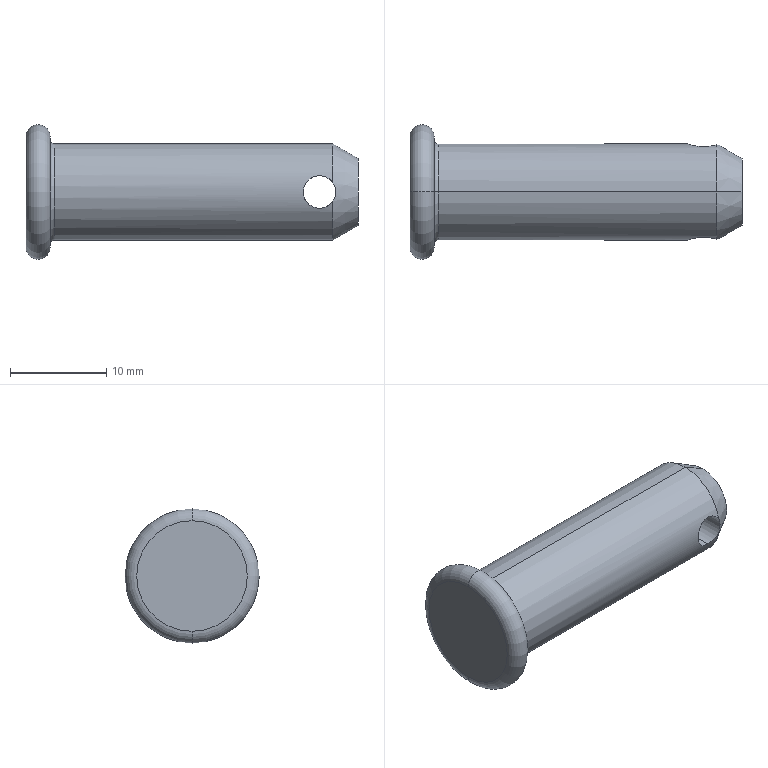Part | SolidWorks | features Chamfer 1, Cut 1, Fillet 1, Revolution 1 | 1 solid | 13 faces | box 34.5 x 14 x 14 mm | volume 2728 mm3 | cylinder 4 | torus 4 | plane 3 | cone 2 | commonest cylinder face diameters 3.38 x2 10 x2
STEP:
#1=CARTESIAN_POINT('',(30.5,-4.706,-1.69));
#2=VERTEX_POINT('',#1);
#3=CARTESIAN_POINT('',(30.5,-4.706,1.69));
#4=VERTEX_POINT('',#3);
#5=CARTESIAN_POINT('',(30.5,-4.706,-1.69));
#6=CARTESIAN_POINT('',(30.276,-4.706,-1.69));
#7=CARTESIAN_POINT('',(30.055,-4.722,-1.645));
#8=CARTESIAN_POINT('',(29.747,-4.765,-1.517));
#9=CARTESIAN_POINT('',(29.65,-4.781,-1.465));
#10=CARTESIAN_POINT('',(29.468,-4.817,-1.343));
#11=CARTESIAN_POINT('',(29.382,-4.836,-1.272));
#12=CARTESIAN_POINT('',(29.15,-4.893,-1.039));
#13=CARTESIAN_POINT('',(29.024,-4.931,-0.8522));
#14=CARTESIAN_POINT('',(28.855,-4.984,-0.4461));
#15=CARTESIAN_POINT('',(28.81,-5.,-0.2222));
#16=CARTESIAN_POINT('',(28.81,-5.,0.1106));
#17=CARTESIAN_POINT('',(28.821,-4.996,0.2234));
#18=CARTESIAN_POINT('',(28.865,-4.982,0.4413));
#19=CARTESIAN_POINT('',(28.897,-4.971,0.547));
#20=CARTESIAN_POINT('',(29.025,-4.931,0.8543));
#21=CARTESIAN_POINT('',(29.149,-4.893,1.04));
#22=CARTESIAN_POINT('',(29.384,-4.836,1.274));
#23=CARTESIAN_POINT('',(29.468,-4.817,1.343));
#24=CARTESIAN_POINT('',(29.65,-4.781,1.465));
#25=CARTESIAN_POINT('',(29.749,-4.764,1.518));
#26=CARTESIAN_POINT('',(29.953,-4.736,1.603));
#27=CARTESIAN_POINT('',(30.058,-4.725,1.635));
#28=CARTESIAN_POINT('',(30.276,-4.71,1.679));
#29=CARTESIAN_POINT('',(30.389,-4.706,1.69));
#30=CARTESIAN_POINT('',(30.5,-4.706,1.69));
#31=B_SPLINE_CURVE_WITH_KNOTS('',3,(#5,#6,#7,#8,#9,#10,#11,#12,#13,#14,#15,#16,#17,#18,#19,#20,#21,#22,#23,#24,#25,#26,#27,#28,#29,#30),.UNSPECIFIED.,.F.,.F.,(4,2,2,2,2,2,2,2,2,2,2,2,4),(0.001661,0.002326,0.002659,0.002992,0.003657,0.004322,0.004654,0.004987,0.005652,0.005985,0.006317,0.00665,0.006982),.UNSPECIFIED.);
#32=EDGE_CURVE('',#2,#4,#31,.T.);
#33=ORIENTED_EDGE('',*,*,#32,.F.);
#34=CARTESIAN_POINT('',(30.5,4.706,-1.69));
#35=VERTEX_POINT('',#34);
#36=CARTESIAN_POINT('',(30.5,-500.,-1.69));
#37=DIRECTION('',(0.,1.,0.));
#38=VECTOR('',#37,1000.);
#39=LINE('',#36,#38);
#40=EDGE_CURVE('',#2,#35,#39,.T.);
#41=ORIENTED_EDGE('',*,*,#40,.T.);
#42=CARTESIAN_POINT('',(30.5,4.706,1.69));
#43=VERTEX_POINT('',#42);
#44=CARTESIAN_POINT('',(30.5,4.706,1.69));
#45=CARTESIAN_POINT('',(30.276,4.706,1.69));
#46=CARTESIAN_POINT('',(30.055,4.722,1.645));
#47=CARTESIAN_POINT('',(29.747,4.765,1.517));
#48=CARTESIAN_POINT('',(29.65,4.781,1.465));
#49=CARTESIAN_POINT('',(29.468,4.817,1.343));
#50=CARTESIAN_POINT('',(29.382,4.836,1.272));
#51=CARTESIAN_POINT('',(29.15,4.893,1.039));
#52=CARTESIAN_POINT('',(29.024,4.931,0.8522));
#53=CARTESIAN_POINT('',(28.855,4.984,0.4461));
#54=CARTESIAN_POINT('',(28.81,5.,0.2222));
#55=CARTESIAN_POINT('',(28.81,5.,-0.1106));
#56=CARTESIAN_POINT('',(28.821,4.996,-0.2234));
#57=CARTESIAN_POINT('',(28.865,4.982,-0.4413));
#58=CARTESIAN_POINT('',(28.897,4.971,-0.547));
#59=CARTESIAN_POINT('',(29.025,4.931,-0.8543));
#60=CARTESIAN_POINT('',(29.149,4.893,-1.04));
#61=CARTESIAN_POINT('',(29.384,4.836,-1.274));
#62=CARTESIAN_POINT('',(29.468,4.817,-1.343));
#63=CARTESIAN_POINT('',(29.65,4.781,-1.465));
#64=CARTESIAN_POINT('',(29.749,4.764,-1.518));
#65=CARTESIAN_POINT('',(29.953,4.736,-1.603));
#66=CARTESIAN_POINT('',(30.058,4.725,-1.635));
#67=CARTESIAN_POINT('',(30.276,4.71,-1.679));
#68=CARTESIAN_POINT('',(30.389,4.706,-1.69));
#69=CARTESIAN_POINT('',(30.5,4.706,-1.69));
#70=B_SPLINE_CURVE_WITH_KNOTS('',3,(#44,#45,#46,#47,#48,#49,#50,#51,#52,#53,#54,#55,#56,#57,#58,#59,#60,#61,#62,#63,#64,#65,#66,#67,#68,#69),.UNSPECIFIED.,.F.,.F.,(4,2,2,2,2,2,2,2,2,2,2,2,4),(0.001661,0.002326,0.002659,0.002992,0.003657,0.004322,0.004654,0.004987,0.005652,0.005985,0.006317,0.00665,0.006982),.UNSPECIFIED.);
#71=EDGE_CURVE('',#43,#35,#70,.T.);
#72=ORIENTED_EDGE('',*,*,#71,.F.);
#73=CARTESIAN_POINT('',(30.5,-500.,1.69));
#74=DIRECTION('',(0.,1.,0.));
#75=VECTOR('',#74,1000.);
#76=LINE('',#73,#75);
#77=EDGE_CURVE('',#4,#43,#76,.T.);
#78=ORIENTED_EDGE('',*,*,#77,.F.);
#79=EDGE_LOOP('',(#33,#41,#72,#78));
#80=FACE_OUTER_BOUND('',#79,.T.);
#81=CARTESIAN_POINT('',(30.5,-500.,0.));
#82=DIRECTION('',(0.,1.,0.));
#83=DIRECTION('',(0.,0.,1.));
#84=AXIS2_PLACEMENT_3D('',#81,#82,#83);
#85=CYLINDRICAL_SURFACE('',#84,1.69);
#86=ADVANCED_FACE('',(#80),#85,.F.);
#87=CARTESIAN_POINT('',(34.5,0.,-3.5));
#88=VERTEX_POINT('',#87);
#89=CARTESIAN_POINT('',(34.5,0.,3.5));
#90=VERTEX_POINT('',#89);
#91=CARTESIAN_POINT('',(34.5,0.,0.));
#92=DIRECTION('',(1.,0.,0.));
#93=DIRECTION('',(0.,0.,1.));
#94=AXIS2_PLACEMENT_3D('',#91,#92,#93);
#95=CIRCLE('',#94,3.5);
#96=EDGE_CURVE('',#88,#90,#95,.T.);
#97=ORIENTED_EDGE('',*,*,#96,.F.);
#98=CARTESIAN_POINT('',(31.902,0.,-5.));
#99=VERTEX_POINT('',#98);
#100=CARTESIAN_POINT('',(31.902,0.,-5.));
#101=DIRECTION('',(-0.866,0.,-0.5));
#102=VECTOR('',#101,1000.);
#103=LINE('',#100,#102);
#104=EDGE_CURVE('',#88,#99,#103,.T.);
#105=ORIENTED_EDGE('',*,*,#104,.T.);
#106=CARTESIAN_POINT('',(31.902,4.91,-0.9438));
#107=VERTEX_POINT('',#106);
#108=CARTESIAN_POINT('',(31.902,0.,0.));
#109=DIRECTION('',(-1.,0.,0.));
#110=DIRECTION('',(0.,0.,1.));
#111=AXIS2_PLACEMENT_3D('',#108,#109,#110);
#112=CIRCLE('',#111,5.);
#113=EDGE_CURVE('',#107,#99,#112,.T.);
#114=ORIENTED_EDGE('',*,*,#113,.F.);
#115=CARTESIAN_POINT('',(31.902,4.91,0.9438));
#116=VERTEX_POINT('',#115);
#117=CARTESIAN_POINT('',(31.902,4.91,0.9438));
#118=CARTESIAN_POINT('',(31.995,4.882,0.8061));
#119=CARTESIAN_POINT('',(32.066,4.864,0.6567));
#120=CARTESIAN_POINT('',(32.165,4.839,0.3342));
#121=CARTESIAN_POINT('',(32.19,4.834,0.1694));
#122=CARTESIAN_POINT('',(32.19,4.834,-0.1673));
#123=CARTESIAN_POINT('',(32.165,4.839,-0.3337));
#124=CARTESIAN_POINT('',(32.067,4.863,-0.6536));
#125=CARTESIAN_POINT('',(31.995,4.882,-0.806));
#126=CARTESIAN_POINT('',(31.902,4.91,-0.9438));
#127=B_SPLINE_CURVE_WITH_KNOTS('',3,(#117,#118,#119,#120,#121,#122,#123,#124,#125,#126),.UNSPECIFIED.,.F.,.F.,(4,2,2,2,4),(0.00005098,0.0005511,0.001051,0.001551,0.002051),.UNSPECIFIED.);
#128=EDGE_CURVE('',#116,#107,#127,.T.);
#129=ORIENTED_EDGE('',*,*,#128,.F.);
#130=CARTESIAN_POINT('',(31.902,0.,5.));
#131=VERTEX_POINT('',#130);
#132=CARTESIAN_POINT('',(31.902,0.,0.));
#133=DIRECTION('',(-1.,0.,0.));
#134=DIRECTION('',(0.,0.,1.));
#135=AXIS2_PLACEMENT_3D('',#132,#133,#134);
#136=CIRCLE('',#135,5.);
#137=EDGE_CURVE('',#131,#116,#136,.T.);
#138=ORIENTED_EDGE('',*,*,#137,.F.);
#139=CARTESIAN_POINT('',(31.902,0.,5.));
#140=DIRECTION('',(-0.866,0.,0.5));
#141=VECTOR('',#140,1000.);
#142=LINE('',#139,#141);
#143=EDGE_CURVE('',#90,#131,#142,.T.);
#144=ORIENTED_EDGE('',*,*,#143,.F.);
#145=EDGE_LOOP('',(#97,#105,#114,#129,#138,#144));
#146=FACE_OUTER_BOUND('',#145,.T.);
#147=CARTESIAN_POINT('',(31.902,0.,0.));
#148=DIRECTION('',(-1.,0.,0.));
#149=DIRECTION('',(0.,0.,1.));
#150=AXIS2_PLACEMENT_3D('',#147,#148,#149);
#151=CONICAL_SURFACE('',#150,5.,0.5236);
#152=ADVANCED_FACE('',(#146),#151,.T.);
#153=CARTESIAN_POINT('',(2.5,0.,-5.5));
#154=VERTEX_POINT('',#153);
#155=CARTESIAN_POINT('',(2.5,0.,5.5));
#156=VERTEX_POINT('',#155);
#157=CARTESIAN_POINT('',(2.5,0.,0.));
#158=DIRECTION('',(-1.,0.,0.));
#159=DIRECTION('',(0.,0.,1.));
#160=AXIS2_PLACEMENT_3D('',#157,#158,#159);
#161=CIRCLE('',#160,5.5);
#162=EDGE_CURVE('',#154,#156,#161,.T.);
#163=ORIENTED_EDGE('',*,*,#162,.F.);
#164=CARTESIAN_POINT('',(3.,0.,-5.));
#165=VERTEX_POINT('',#164);
#166=CARTESIAN_POINT('',(3.,0.,-5.5));
#167=DIRECTION('',(0.,1.,0.));
#168=DIRECTION('',(0.,0.,1.));
#169=AXIS2_PLACEMENT_3D('',#166,#167,#168);
#170=CIRCLE('',#169,0.5);
#171=EDGE_CURVE('',#154,#165,#170,.T.);
#172=ORIENTED_EDGE('',*,*,#171,.T.);
#173=CARTESIAN_POINT('',(3.,0.,5.));
#174=VERTEX_POINT('',#173);
#175=CARTESIAN_POINT('',(3.,0.,0.));
#176=DIRECTION('',(1.,0.,0.));
#177=DIRECTION('',(0.,0.,1.));
#178=AXIS2_PLACEMENT_3D('',#175,#176,#177);
#179=CIRCLE('',#178,5.);
#180=EDGE_CURVE('',#174,#165,#179,.T.);
#181=ORIENTED_EDGE('',*,*,#180,.F.);
#182=CARTESIAN_POINT('',(3.,0.,5.5));
#183=DIRECTION('',(0.,-1.,0.));
#184=DIRECTION('',(0.,0.,-1.));
#185=AXIS2_PLACEMENT_3D('',#182,#183,#184);
#186=CIRCLE('',#185,0.5);
#187=EDGE_CURVE('',#156,#174,#186,.T.);
#188=ORIENTED_EDGE('',*,*,#187,.F.);
#189=EDGE_LOOP('',(#163,#172,#181,#188));
#190=FACE_OUTER_BOUND('',#189,.T.);
#191=CARTESIAN_POINT('',(3.,0.,0.));
#192=DIRECTION('',(-1.,0.,0.));
#193=DIRECTION('',(0.,0.,1.));
#194=AXIS2_PLACEMENT_3D('',#191,#192,#193);
#195=TOROIDAL_SURFACE('',#194,5.5,0.5);
#196=ADVANCED_FACE('',(#190),#195,.F.);
#197=ORIENTED_EDGE('',*,*,#113,.T.);
#198=CARTESIAN_POINT('',(0.,0.,-5.));
#199=DIRECTION('',(-1.,0.,0.));
#200=VECTOR('',#199,1000.);
#201=LINE('',#198,#200);
#202=EDGE_CURVE('',#99,#165,#201,.T.);
#203=ORIENTED_EDGE('',*,*,#202,.T.);
#204=CARTESIAN_POINT('',(3.,0.,0.));
#205=DIRECTION('',(1.,0.,0.));
#206=DIRECTION('',(0.,0.,1.));
#207=AXIS2_PLACEMENT_3D('',#204,#205,#206);
#208=CIRCLE('',#207,5.);
#209=EDGE_CURVE('',#165,#174,#208,.T.);
#210=ORIENTED_EDGE('',*,*,#209,.T.);
#211=CARTESIAN_POINT('',(0.,0.,5.));
#212=DIRECTION('',(-1.,0.,0.));
#213=VECTOR('',#212,1000.);
#214=LINE('',#211,#213);
#215=EDGE_CURVE('',#131,#174,#214,.T.);
#216=ORIENTED_EDGE('',*,*,#215,.F.);
#217=ORIENTED_EDGE('',*,*,#137,.T.);
#218=CARTESIAN_POINT('',(31.902,4.91,0.9438));
#219=CARTESIAN_POINT('',(31.824,4.888,1.059));
#220=CARTESIAN_POINT('',(31.735,4.864,1.162));
#221=CARTESIAN_POINT('',(31.532,4.817,1.345));
#222=CARTESIAN_POINT('',(31.418,4.793,1.426));
#223=CARTESIAN_POINT('',(31.176,4.753,1.555));
#224=CARTESIAN_POINT('',(31.046,4.735,1.605));
#225=CARTESIAN_POINT('',(30.777,4.712,1.673));
#226=CARTESIAN_POINT('',(30.64,4.706,1.69));
#227=CARTESIAN_POINT('',(30.5,4.706,1.69));
#228=B_SPLINE_CURVE_WITH_KNOTS('',3,(#218,#219,#220,#221,#222,#223,#224,#225,#226,#227),.UNSPECIFIED.,.F.,.F.,(4,2,2,2,4),(0.,0.0004153,0.0008306,0.001246,0.001661),.UNSPECIFIED.);
#229=EDGE_CURVE('',#116,#43,#228,.T.);
#230=ORIENTED_EDGE('',*,*,#229,.T.);
#231=ORIENTED_EDGE('',*,*,#71,.T.);
#232=CARTESIAN_POINT('',(30.5,4.706,-1.69));
#233=CARTESIAN_POINT('',(30.638,4.706,-1.69));
#234=CARTESIAN_POINT('',(30.777,4.712,-1.673));
#235=CARTESIAN_POINT('',(31.047,4.735,-1.605));
#236=CARTESIAN_POINT('',(31.175,4.752,-1.556));
#237=CARTESIAN_POINT('',(31.54,4.813,-1.36));
#238=CARTESIAN_POINT('',(31.747,4.866,-1.173));
#239=CARTESIAN_POINT('',(31.902,4.91,-0.9438));
#240=B_SPLINE_CURVE_WITH_KNOTS('',3,(#232,#233,#234,#235,#236,#237,#238,#239),.UNSPECIFIED.,.F.,.F.,(4,2,2,4),(0.006982,0.007397,0.007811,0.00864),.UNSPECIFIED.);
#241=EDGE_CURVE('',#35,#107,#240,.T.);
#242=ORIENTED_EDGE('',*,*,#241,.T.);
#243=EDGE_LOOP('',(#197,#203,#210,#216,#217,#230,#231,#242));
#244=FACE_OUTER_BOUND('',#243,.T.);
#245=CARTESIAN_POINT('',(0.,0.,0.));
#246=DIRECTION('',(-1.,0.,0.));
#247=DIRECTION('',(0.,0.,1.));
#248=AXIS2_PLACEMENT_3D('',#245,#246,#247);
#249=CYLINDRICAL_SURFACE('',#248,5.);
#250=ADVANCED_FACE('',(#244),#249,.T.);
#251=CARTESIAN_POINT('',(2.5,0.,5.75));
#252=VERTEX_POINT('',#251);
#253=CARTESIAN_POINT('',(2.5,0.,-5.75));
#254=VERTEX_POINT('',#253);
#255=CARTESIAN_POINT('',(2.5,0.,0.));
#256=DIRECTION('',(-1.,0.,0.));
#257=DIRECTION('',(0.,0.,1.));
#258=AXIS2_PLACEMENT_3D('',#255,#256,#257);
#259=CIRCLE('',#258,5.75);
#260=EDGE_CURVE('',#252,#254,#259,.T.);
#261=ORIENTED_EDGE('',*,*,#260,.T.);
#262=CARTESIAN_POINT('',(0.,0.,-5.75));
#263=VERTEX_POINT('',#262);
#264=CARTESIAN_POINT('',(1.25,0.,-5.75));
#265=DIRECTION('',(0.,1.,0.));
#266=DIRECTION('',(0.,0.,1.));
#267=AXIS2_PLACEMENT_3D('',#264,#265,#266);
#268=CIRCLE('',#267,1.25);
#269=EDGE_CURVE('',#254,#263,#268,.T.);
#270=ORIENTED_EDGE('',*,*,#269,.T.);
#271=CARTESIAN_POINT('',(0.,0.,5.75));
#272=VERTEX_POINT('',#271);
#273=CARTESIAN_POINT('',(0.,0.,0.));
#274=DIRECTION('',(-1.,0.,0.));
#275=DIRECTION('',(0.,0.,1.));
#276=AXIS2_PLACEMENT_3D('',#273,#274,#275);
#277=CIRCLE('',#276,5.75);
#278=EDGE_CURVE('',#272,#263,#277,.T.);
#279=ORIENTED_EDGE('',*,*,#278,.F.);
#280=CARTESIAN_POINT('',(1.25,0.,5.75));
#281=DIRECTION('',(0.,-1.,0.));
#282=DIRECTION('',(0.,0.,-1.));
#283=AXIS2_PLACEMENT_3D('',#280,#281,#282);
#284=CIRCLE('',#283,1.25);
#285=EDGE_CURVE('',#252,#272,#284,.T.);
#286=ORIENTED_EDGE('',*,*,#285,.F.);
#287=EDGE_LOOP('',(#261,#270,#279,#286));
#288=FACE_OUTER_BOUND('',#287,.T.);
#289=CARTESIAN_POINT('',(1.25,0.,0.));
#290=DIRECTION('',(-1.,0.,0.));
#291=DIRECTION('',(0.,0.,1.));
#292=AXIS2_PLACEMENT_3D('',#289,#290,#291);
#293=TOROIDAL_SURFACE('',#292,5.75,1.25);
#294=ADVANCED_FACE('',(#288),#293,.T.);
#295=ORIENTED_EDGE('',*,*,#278,.T.);
#296=CARTESIAN_POINT('',(0.,0.,0.));
#297=DIRECTION('',(-1.,0.,0.));
#298=DIRECTION('',(0.,0.,1.));
#299=AXIS2_PLACEMENT_3D('',#296,#297,#298);
#300=CIRCLE('',#299,5.75);
#301=EDGE_CURVE('',#263,#272,#300,.T.);
#302=ORIENTED_EDGE('',*,*,#301,.T.);
#303=EDGE_LOOP('',(#295,#302));
#304=FACE_OUTER_BOUND('',#303,.T.);
#305=CARTESIAN_POINT('',(0.,0.,0.));
#306=DIRECTION('',(1.,0.,0.));
#307=DIRECTION('',(0.,0.,-1.));
#308=AXIS2_PLACEMENT_3D('',#305,#306,#307);
#309=PLANE('',#308);
#310=ADVANCED_FACE('',(#304),#309,.F.);
#311=ORIENTED_EDGE('',*,*,#269,.F.);
#312=CARTESIAN_POINT('',(2.5,0.,0.));
#313=DIRECTION('',(-1.,0.,0.));
#314=DIRECTION('',(0.,0.,1.));
#315=AXIS2_PLACEMENT_3D('',#312,#313,#314);
#316=CIRCLE('',#315,5.75);
#317=EDGE_CURVE('',#254,#252,#316,.T.);
#318=ORIENTED_EDGE('',*,*,#317,.T.);
#319=ORIENTED_EDGE('',*,*,#285,.T.);
#320=ORIENTED_EDGE('',*,*,#301,.F.);
#321=EDGE_LOOP('',(#311,#318,#319,#320));
#322=FACE_OUTER_BOUND('',#321,.T.);
#323=CARTESIAN_POINT('',(1.25,0.,0.));
#324=DIRECTION('',(-1.,0.,0.));
#325=DIRECTION('',(0.,0.,1.));
#326=AXIS2_PLACEMENT_3D('',#323,#324,#325);
#327=TOROIDAL_SURFACE('',#326,5.75,1.25);
#328=ADVANCED_FACE('',(#322),#327,.T.);
#329=CARTESIAN_POINT('',(2.5,0.,0.));
#330=DIRECTION('',(-1.,0.,0.));
#331=DIRECTION('',(0.,0.,1.));
#332=AXIS2_PLACEMENT_3D('',#329,#330,#331);
#333=CIRCLE('',#332,5.5);
#334=EDGE_CURVE('',#156,#154,#333,.T.);
#335=ORIENTED_EDGE('',*,*,#334,.T.);
#336=ORIENTED_EDGE('',*,*,#162,.T.);
#337=EDGE_LOOP('',(#335,#336));
#338=FACE_BOUND('',#337,.T.);
#339=ORIENTED_EDGE('',*,*,#260,.F.);
#340=ORIENTED_EDGE('',*,*,#317,.F.);
#341=EDGE_LOOP('',(#339,#340));
#342=FACE_OUTER_BOUND('',#341,.T.);
#343=CARTESIAN_POINT('',(2.5,5.75,0.));
#344=DIRECTION('',(-1.,0.,0.));
#345=DIRECTION('',(0.,0.,1.));
#346=AXIS2_PLACEMENT_3D('',#343,#344,#345);
#347=PLANE('',#346);
#348=ADVANCED_FACE('',(#338,#342),#347,.F.);
#349=ORIENTED_EDGE('',*,*,#202,.F.);
#350=CARTESIAN_POINT('',(31.902,-4.91,-0.9438));
#351=VERTEX_POINT('',#350);
#352=CARTESIAN_POINT('',(31.902,0.,0.));
#353=DIRECTION('',(-1.,0.,0.));
#354=DIRECTION('',(0.,0.,1.));
#355=AXIS2_PLACEMENT_3D('',#352,#353,#354);
#356=CIRCLE('',#355,5.);
#357=EDGE_CURVE('',#99,#351,#356,.T.);
#358=ORIENTED_EDGE('',*,*,#357,.T.);
#359=CARTESIAN_POINT('',(31.902,-4.91,-0.9438));
#360=CARTESIAN_POINT('',(31.824,-4.888,-1.059));
#361=CARTESIAN_POINT('',(31.735,-4.864,-1.162));
#362=CARTESIAN_POINT('',(31.532,-4.817,-1.345));
#363=CARTESIAN_POINT('',(31.418,-4.793,-1.426));
#364=CARTESIAN_POINT('',(31.176,-4.753,-1.555));
#365=CARTESIAN_POINT('',(31.046,-4.735,-1.605));
#366=CARTESIAN_POINT('',(30.777,-4.712,-1.673));
#367=CARTESIAN_POINT('',(30.64,-4.706,-1.69));
#368=CARTESIAN_POINT('',(30.5,-4.706,-1.69));
#369=B_SPLINE_CURVE_WITH_KNOTS('',3,(#359,#360,#361,#362,#363,#364,#365,#366,#367,#368),.UNSPECIFIED.,.F.,.F.,(4,2,2,2,4),(0.,0.0004153,0.0008306,0.001246,0.001661),.UNSPECIFIED.);
#370=EDGE_CURVE('',#351,#2,#369,.T.);
#371=ORIENTED_EDGE('',*,*,#370,.T.);
#372=ORIENTED_EDGE('',*,*,#32,.T.);
#373=CARTESIAN_POINT('',(31.902,-4.91,0.9438));
#374=VERTEX_POINT('',#373);
#375=CARTESIAN_POINT('',(30.5,-4.706,1.69));
#376=CARTESIAN_POINT('',(30.638,-4.706,1.69));
#377=CARTESIAN_POINT('',(30.777,-4.712,1.673));
#378=CARTESIAN_POINT('',(31.047,-4.735,1.605));
#379=CARTESIAN_POINT('',(31.175,-4.752,1.556));
#380=CARTESIAN_POINT('',(31.54,-4.813,1.36));
#381=CARTESIAN_POINT('',(31.747,-4.866,1.173));
#382=CARTESIAN_POINT('',(31.902,-4.91,0.9438));
#383=B_SPLINE_CURVE_WITH_KNOTS('',3,(#375,#376,#377,#378,#379,#380,#381,#382),.UNSPECIFIED.,.F.,.F.,(4,2,2,4),(0.006982,0.007397,0.007811,0.00864),.UNSPECIFIED.);
#384=EDGE_CURVE('',#4,#374,#383,.T.);
#385=ORIENTED_EDGE('',*,*,#384,.T.);
#386=CARTESIAN_POINT('',(31.902,0.,0.));
#387=DIRECTION('',(-1.,0.,0.));
#388=DIRECTION('',(0.,0.,1.));
#389=AXIS2_PLACEMENT_3D('',#386,#387,#388);
#390=CIRCLE('',#389,5.);
#391=EDGE_CURVE('',#374,#131,#390,.T.);
#392=ORIENTED_EDGE('',*,*,#391,.T.);
#393=ORIENTED_EDGE('',*,*,#215,.T.);
#394=ORIENTED_EDGE('',*,*,#180,.T.);
#395=EDGE_LOOP('',(#349,#358,#371,#372,#385,#392,#393,#394));
#396=FACE_OUTER_BOUND('',#395,.T.);
#397=CARTESIAN_POINT('',(0.,0.,0.));
#398=DIRECTION('',(-1.,0.,0.));
#399=DIRECTION('',(0.,0.,1.));
#400=AXIS2_PLACEMENT_3D('',#397,#398,#399);
#401=CYLINDRICAL_SURFACE('',#400,5.);
#402=ADVANCED_FACE('',(#396),#401,.T.);
#403=CARTESIAN_POINT('',(34.5,0.,0.));
#404=DIRECTION('',(1.,0.,0.));
#405=DIRECTION('',(0.,0.,1.));
#406=AXIS2_PLACEMENT_3D('',#403,#404,#405);
#407=CIRCLE('',#406,3.5);
#408=EDGE_CURVE('',#90,#88,#407,.T.);
#409=ORIENTED_EDGE('',*,*,#408,.T.);
#410=ORIENTED_EDGE('',*,*,#96,.T.);
#411=EDGE_LOOP('',(#409,#410));
#412=FACE_OUTER_BOUND('',#411,.T.);
#413=CARTESIAN_POINT('',(34.5,5.,0.));
#414=DIRECTION('',(-1.,0.,0.));
#415=DIRECTION('',(0.,0.,1.));
#416=AXIS2_PLACEMENT_3D('',#413,#414,#415);
#417=PLANE('',#416);
#418=ADVANCED_FACE('',(#412),#417,.F.);
#419=ORIENTED_EDGE('',*,*,#171,.F.);
#420=ORIENTED_EDGE('',*,*,#334,.F.);
#421=ORIENTED_EDGE('',*,*,#187,.T.);
#422=ORIENTED_EDGE('',*,*,#209,.F.);
#423=EDGE_LOOP('',(#419,#420,#421,#422));
#424=FACE_OUTER_BOUND('',#423,.T.);
#425=CARTESIAN_POINT('',(3.,0.,0.));
#426=DIRECTION('',(-1.,0.,0.));
#427=DIRECTION('',(0.,0.,1.));
#428=AXIS2_PLACEMENT_3D('',#425,#426,#427);
#429=TOROIDAL_SURFACE('',#428,5.5,0.5);
#430=ADVANCED_FACE('',(#424),#429,.F.);
#431=ORIENTED_EDGE('',*,*,#104,.F.);
#432=ORIENTED_EDGE('',*,*,#408,.F.);
#433=ORIENTED_EDGE('',*,*,#143,.T.);
#434=ORIENTED_EDGE('',*,*,#391,.F.);
#435=CARTESIAN_POINT('',(31.902,-4.91,-0.9438));
#436=CARTESIAN_POINT('',(31.995,-4.882,-0.8061));
#437=CARTESIAN_POINT('',(32.066,-4.864,-0.6567));
#438=CARTESIAN_POINT('',(32.165,-4.839,-0.3342));
#439=CARTESIAN_POINT('',(32.19,-4.834,-0.1694));
#440=CARTESIAN_POINT('',(32.19,-4.834,0.1673));
#441=CARTESIAN_POINT('',(32.165,-4.839,0.3337));
#442=CARTESIAN_POINT('',(32.067,-4.863,0.6536));
#443=CARTESIAN_POINT('',(31.995,-4.882,0.806));
#444=CARTESIAN_POINT('',(31.902,-4.91,0.9438));
#445=B_SPLINE_CURVE_WITH_KNOTS('',3,(#435,#436,#437,#438,#439,#440,#441,#442,#443,#444),.UNSPECIFIED.,.F.,.F.,(4,2,2,2,4),(0.00005098,0.0005511,0.001051,0.001551,0.002051),.UNSPECIFIED.);
#446=EDGE_CURVE('',#351,#374,#445,.T.);
#447=ORIENTED_EDGE('',*,*,#446,.F.);
#448=ORIENTED_EDGE('',*,*,#357,.F.);
#449=EDGE_LOOP('',(#431,#432,#433,#434,#447,#448));
#450=FACE_OUTER_BOUND('',#449,.T.);
#451=CARTESIAN_POINT('',(31.902,0.,0.));
#452=DIRECTION('',(-1.,0.,0.));
#453=DIRECTION('',(0.,0.,1.));
#454=AXIS2_PLACEMENT_3D('',#451,#452,#453);
#455=CONICAL_SURFACE('',#454,5.,0.5236);
#456=ADVANCED_FACE('',(#450),#455,.T.);
#457=ORIENTED_EDGE('',*,*,#40,.F.);
#458=ORIENTED_EDGE('',*,*,#370,.F.);
#459=ORIENTED_EDGE('',*,*,#446,.T.);
#460=ORIENTED_EDGE('',*,*,#384,.F.);
#461=ORIENTED_EDGE('',*,*,#77,.T.);
#462=ORIENTED_EDGE('',*,*,#229,.F.);
#463=ORIENTED_EDGE('',*,*,#128,.T.);
#464=ORIENTED_EDGE('',*,*,#241,.F.);
#465=EDGE_LOOP('',(#457,#458,#459,#460,#461,#462,#463,#464));
#466=FACE_OUTER_BOUND('',#465,.T.);
#467=CARTESIAN_POINT('',(30.5,-500.,0.));
#468=DIRECTION('',(0.,1.,0.));
#469=DIRECTION('',(0.,0.,1.));
#470=AXIS2_PLACEMENT_3D('',#467,#468,#469);
#471=CYLINDRICAL_SURFACE('',#470,1.69);
#472=ADVANCED_FACE('',(#466),#471,.F.);
#473=CLOSED_SHELL('',(#86,#152,#196,#250,#294,#310,#328,#348,#402,#418,#430,#456,#472));
#474=MANIFOLD_SOLID_BREP('',#473);
#475=CARTESIAN_POINT('',(0.,0.,0.));
#476=DIRECTION('',(0.,0.,1.));
#477=DIRECTION('',(1.,0.,0.));
#478=AXIS2_PLACEMENT_3D('',#475,#476,#477);
#479=(LENGTH_UNIT()NAMED_UNIT(*)SI_UNIT(.MILLI.,.METRE.));
#480=UNCERTAINTY_MEASURE_WITH_UNIT(LENGTH_MEASURE(0.00001),#479,'','');
#481=(NAMED_UNIT(*)PLANE_ANGLE_UNIT()SI_UNIT($,.RADIAN.));
#482=(NAMED_UNIT(*)SI_UNIT($,.STERADIAN.)SOLID_ANGLE_UNIT());
#483=(GEOMETRIC_REPRESENTATION_CONTEXT(3)GLOBAL_UNCERTAINTY_ASSIGNED_CONTEXT((#480))GLOBAL_UNIT_ASSIGNED_CONTEXT((#479,#481,#482))REPRESENTATION_CONTEXT('',''));
#484=ADVANCED_BREP_SHAPE_REPRESENTATION('',(#474,#478),#483);